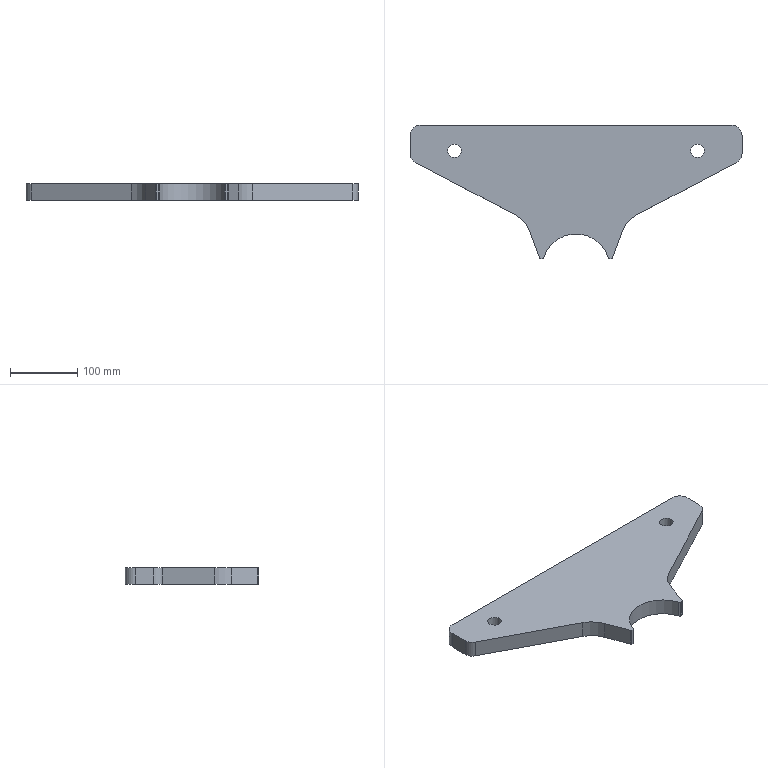Part | NX | features 压板 2 | 1 solid | 24 faces | box 492 x 197.84 x 25 mm | volume 1447958 mm3 | cylinder 13 | plane 11 | commonest cylinder face diameters 4 x4 30 x4 20 x2 90 x2 100 x1
STEP:
#1=CARTESIAN_POINT('',(190.,173.16,25.));
#2=VERTEX_POINT('',#1);
#3=CARTESIAN_POINT('',(180.,173.16,25.));
#4=DIRECTION('',(0.,0.,1.));
#5=DIRECTION('',(1.,0.,0.));
#6=AXIS2_PLACEMENT_3D('',#3,#4,#5);
#7=CIRCLE('',#6,10.);
#8=EDGE_CURVE('',#2,#2,#7,.T.);
#9=ORIENTED_EDGE('',*,*,#8,.F.);
#10=EDGE_LOOP('',(#9));
#11=FACE_BOUND('',#10,.T.);
#12=CARTESIAN_POINT('',(52.393,13.16,25.));
#13=VERTEX_POINT('',#12);
#14=CARTESIAN_POINT('',(54.273,14.476,25.));
#15=VERTEX_POINT('',#14);
#16=CARTESIAN_POINT('',(52.393,15.16,25.));
#17=DIRECTION('',(0.,0.,1.));
#18=DIRECTION('',(-1.,0.,0.));
#19=AXIS2_PLACEMENT_3D('',#16,#17,#18);
#20=CIRCLE('',#19,2.);
#21=EDGE_CURVE('',#13,#15,#20,.T.);
#22=ORIENTED_EDGE('',*,*,#21,.T.);
#23=CARTESIAN_POINT('',(68.526,53.635,25.));
#24=VERTEX_POINT('',#23);
#25=CARTESIAN_POINT('',(54.273,14.476,25.));
#26=DIRECTION('',(0.342,0.9397,0.));
#27=VECTOR('',#26,1000.);
#28=LINE('',#25,#27);
#29=EDGE_CURVE('',#15,#24,#28,.T.);
#30=ORIENTED_EDGE('',*,*,#29,.T.);
#31=CARTESIAN_POINT('',(89.903,78.092,25.));
#32=VERTEX_POINT('',#31);
#33=CARTESIAN_POINT('',(110.812,38.244,25.));
#34=DIRECTION('',(0.,0.,-1.));
#35=DIRECTION('',(-1.,0.,0.));
#36=AXIS2_PLACEMENT_3D('',#33,#34,#35);
#37=CIRCLE('',#36,45.);
#38=EDGE_CURVE('',#24,#32,#37,.T.);
#39=ORIENTED_EDGE('',*,*,#38,.T.);
#40=CARTESIAN_POINT('',(237.97,155.786,25.));
#41=VERTEX_POINT('',#40);
#42=CARTESIAN_POINT('',(237.97,155.786,25.));
#43=DIRECTION('',(0.8855,0.4646,0.));
#44=VECTOR('',#43,1000.);
#45=LINE('',#42,#44);
#46=EDGE_CURVE('',#32,#41,#45,.T.);
#47=ORIENTED_EDGE('',*,*,#46,.T.);
#48=CARTESIAN_POINT('',(246.,169.069,25.));
#49=VERTEX_POINT('',#48);
#50=CARTESIAN_POINT('',(231.,169.069,25.));
#51=DIRECTION('',(0.,0.,1.));
#52=DIRECTION('',(1.,0.,0.));
#53=AXIS2_PLACEMENT_3D('',#50,#51,#52);
#54=CIRCLE('',#53,15.);
#55=EDGE_CURVE('',#41,#49,#54,.T.);
#56=ORIENTED_EDGE('',*,*,#55,.T.);
#57=CARTESIAN_POINT('',(246.,196.,25.));
#58=VERTEX_POINT('',#57);
#59=CARTESIAN_POINT('',(246.,196.,25.));
#60=DIRECTION('',(0.,1.,0.));
#61=VECTOR('',#60,1000.);
#62=LINE('',#59,#61);
#63=EDGE_CURVE('',#49,#58,#62,.T.);
#64=ORIENTED_EDGE('',*,*,#63,.T.);
#65=CARTESIAN_POINT('',(231.,211.,25.));
#66=VERTEX_POINT('',#65);
#67=CARTESIAN_POINT('',(231.,196.,25.));
#68=DIRECTION('',(0.,0.,1.));
#69=DIRECTION('',(1.,0.,0.));
#70=AXIS2_PLACEMENT_3D('',#67,#68,#69);
#71=CIRCLE('',#70,15.);
#72=EDGE_CURVE('',#58,#66,#71,.T.);
#73=ORIENTED_EDGE('',*,*,#72,.T.);
#74=CARTESIAN_POINT('',(-231.,211.,25.));
#75=VERTEX_POINT('',#74);
#76=CARTESIAN_POINT('',(231.,211.,25.));
#77=DIRECTION('',(-1.,0.,0.));
#78=VECTOR('',#77,1000.);
#79=LINE('',#76,#78);
#80=EDGE_CURVE('',#66,#75,#79,.T.);
#81=ORIENTED_EDGE('',*,*,#80,.T.);
#82=CARTESIAN_POINT('',(-246.,196.,25.));
#83=VERTEX_POINT('',#82);
#84=CARTESIAN_POINT('',(-231.,196.,25.));
#85=DIRECTION('',(0.,0.,1.));
#86=DIRECTION('',(-1.,0.,0.));
#87=AXIS2_PLACEMENT_3D('',#84,#85,#86);
#88=CIRCLE('',#87,15.);
#89=EDGE_CURVE('',#75,#83,#88,.T.);
#90=ORIENTED_EDGE('',*,*,#89,.T.);
#91=CARTESIAN_POINT('',(-246.,169.069,25.));
#92=VERTEX_POINT('',#91);
#93=CARTESIAN_POINT('',(-246.,196.,25.));
#94=DIRECTION('',(0.,-1.,0.));
#95=VECTOR('',#94,1000.);
#96=LINE('',#93,#95);
#97=EDGE_CURVE('',#83,#92,#96,.T.);
#98=ORIENTED_EDGE('',*,*,#97,.T.);
#99=CARTESIAN_POINT('',(-237.97,155.786,25.));
#100=VERTEX_POINT('',#99);
#101=CARTESIAN_POINT('',(-231.,169.069,25.));
#102=DIRECTION('',(0.,0.,1.));
#103=DIRECTION('',(-1.,0.,0.));
#104=AXIS2_PLACEMENT_3D('',#101,#102,#103);
#105=CIRCLE('',#104,15.);
#106=EDGE_CURVE('',#92,#100,#105,.T.);
#107=ORIENTED_EDGE('',*,*,#106,.T.);
#108=CARTESIAN_POINT('',(-89.903,78.092,25.));
#109=VERTEX_POINT('',#108);
#110=CARTESIAN_POINT('',(-237.97,155.786,25.));
#111=DIRECTION('',(0.8855,-0.4646,0.));
#112=VECTOR('',#111,1000.);
#113=LINE('',#110,#112);
#114=EDGE_CURVE('',#100,#109,#113,.T.);
#115=ORIENTED_EDGE('',*,*,#114,.T.);
#116=CARTESIAN_POINT('',(-68.526,53.635,25.));
#117=VERTEX_POINT('',#116);
#118=CARTESIAN_POINT('',(-110.812,38.244,25.));
#119=DIRECTION('',(0.,0.,-1.));
#120=DIRECTION('',(1.,0.,0.));
#121=AXIS2_PLACEMENT_3D('',#118,#119,#120);
#122=CIRCLE('',#121,45.);
#123=EDGE_CURVE('',#109,#117,#122,.T.);
#124=ORIENTED_EDGE('',*,*,#123,.T.);
#125=CARTESIAN_POINT('',(-54.273,14.476,25.));
#126=VERTEX_POINT('',#125);
#127=CARTESIAN_POINT('',(-54.273,14.476,25.));
#128=DIRECTION('',(0.342,-0.9397,0.));
#129=VECTOR('',#128,1000.);
#130=LINE('',#127,#129);
#131=EDGE_CURVE('',#117,#126,#130,.T.);
#132=ORIENTED_EDGE('',*,*,#131,.T.);
#133=CARTESIAN_POINT('',(-52.393,13.16,25.));
#134=VERTEX_POINT('',#133);
#135=CARTESIAN_POINT('',(-52.393,15.16,25.));
#136=DIRECTION('',(0.,0.,1.));
#137=DIRECTION('',(1.,0.,0.));
#138=AXIS2_PLACEMENT_3D('',#135,#136,#137);
#139=CIRCLE('',#138,2.);
#140=EDGE_CURVE('',#126,#134,#139,.T.);
#141=ORIENTED_EDGE('',*,*,#140,.T.);
#142=CARTESIAN_POINT('',(-49.741,13.16,25.));
#143=VERTEX_POINT('',#142);
#144=CARTESIAN_POINT('',(-49.741,13.16,25.));
#145=DIRECTION('',(1.,0.,0.));
#146=VECTOR('',#145,1000.);
#147=LINE('',#144,#146);
#148=EDGE_CURVE('',#134,#143,#147,.T.);
#149=ORIENTED_EDGE('',*,*,#148,.T.);
#150=CARTESIAN_POINT('',(-47.828,14.577,25.));
#151=VERTEX_POINT('',#150);
#152=CARTESIAN_POINT('',(-49.741,15.16,25.));
#153=DIRECTION('',(0.,0.,1.));
#154=DIRECTION('',(1.,0.,0.));
#155=AXIS2_PLACEMENT_3D('',#152,#153,#154);
#156=CIRCLE('',#155,2.);
#157=EDGE_CURVE('',#143,#151,#156,.T.);
#158=ORIENTED_EDGE('',*,*,#157,.T.);
#159=CARTESIAN_POINT('',(47.828,14.577,25.));
#160=VERTEX_POINT('',#159);
#161=CARTESIAN_POINT('',(0.,0.,25.));
#162=DIRECTION('',(0.,0.,-1.));
#163=DIRECTION('',(1.,0.,0.));
#164=AXIS2_PLACEMENT_3D('',#161,#162,#163);
#165=CIRCLE('',#164,50.);
#166=EDGE_CURVE('',#151,#160,#165,.T.);
#167=ORIENTED_EDGE('',*,*,#166,.T.);
#168=CARTESIAN_POINT('',(49.741,13.16,25.));
#169=VERTEX_POINT('',#168);
#170=CARTESIAN_POINT('',(49.741,15.16,25.));
#171=DIRECTION('',(0.,0.,1.));
#172=DIRECTION('',(-1.,0.,0.));
#173=AXIS2_PLACEMENT_3D('',#170,#171,#172);
#174=CIRCLE('',#173,2.);
#175=EDGE_CURVE('',#160,#169,#174,.T.);
#176=ORIENTED_EDGE('',*,*,#175,.T.);
#177=CARTESIAN_POINT('',(49.741,13.16,25.));
#178=DIRECTION('',(1.,0.,0.));
#179=VECTOR('',#178,1000.);
#180=LINE('',#177,#179);
#181=EDGE_CURVE('',#169,#13,#180,.T.);
#182=ORIENTED_EDGE('',*,*,#181,.T.);
#183=EDGE_LOOP('',(#22,#30,#39,#47,#56,#64,#73,#81,#90,#98,#107,#115,#124,#132,#141,#149,#158,#167,#176,#182));
#184=FACE_BOUND('',#183,.T.);
#185=CARTESIAN_POINT('',(-190.,173.16,25.));
#186=VERTEX_POINT('',#185);
#187=CARTESIAN_POINT('',(-180.,173.16,25.));
#188=DIRECTION('',(0.,0.,1.));
#189=DIRECTION('',(-1.,0.,0.));
#190=AXIS2_PLACEMENT_3D('',#187,#188,#189);
#191=CIRCLE('',#190,10.);
#192=EDGE_CURVE('',#186,#186,#191,.T.);
#193=ORIENTED_EDGE('',*,*,#192,.F.);
#194=EDGE_LOOP('',(#193));
#195=FACE_BOUND('',#194,.T.);
#196=CARTESIAN_POINT('',(52.393,15.16,25.));
#197=DIRECTION('',(0.,0.,-1.));
#198=DIRECTION('',(-1.,0.,0.));
#199=AXIS2_PLACEMENT_3D('',#196,#197,#198);
#200=PLANE('',#199);
#201=ADVANCED_FACE('',(#11,#184,#195),#200,.F.);
#202=CARTESIAN_POINT('',(190.,173.16,0.));
#203=VERTEX_POINT('',#202);
#204=CARTESIAN_POINT('',(180.,173.16,0.));
#205=DIRECTION('',(0.,0.,1.));
#206=DIRECTION('',(1.,0.,0.));
#207=AXIS2_PLACEMENT_3D('',#204,#205,#206);
#208=CIRCLE('',#207,10.);
#209=EDGE_CURVE('',#203,#203,#208,.T.);
#210=ORIENTED_EDGE('',*,*,#209,.T.);
#211=EDGE_LOOP('',(#210));
#212=FACE_BOUND('',#211,.T.);
#213=CARTESIAN_POINT('',(52.393,13.16,0.));
#214=VERTEX_POINT('',#213);
#215=CARTESIAN_POINT('',(54.273,14.476,0.));
#216=VERTEX_POINT('',#215);
#217=CARTESIAN_POINT('',(52.393,15.16,0.));
#218=DIRECTION('',(0.,0.,1.));
#219=DIRECTION('',(-1.,0.,0.));
#220=AXIS2_PLACEMENT_3D('',#217,#218,#219);
#221=CIRCLE('',#220,2.);
#222=EDGE_CURVE('',#214,#216,#221,.T.);
#223=ORIENTED_EDGE('',*,*,#222,.F.);
#224=CARTESIAN_POINT('',(49.741,13.16,0.));
#225=VERTEX_POINT('',#224);
#226=CARTESIAN_POINT('',(49.741,13.16,0.));
#227=DIRECTION('',(1.,0.,0.));
#228=VECTOR('',#227,1000.);
#229=LINE('',#226,#228);
#230=EDGE_CURVE('',#225,#214,#229,.T.);
#231=ORIENTED_EDGE('',*,*,#230,.F.);
#232=CARTESIAN_POINT('',(47.828,14.577,0.));
#233=VERTEX_POINT('',#232);
#234=CARTESIAN_POINT('',(49.741,15.16,0.));
#235=DIRECTION('',(0.,0.,1.));
#236=DIRECTION('',(-1.,0.,0.));
#237=AXIS2_PLACEMENT_3D('',#234,#235,#236);
#238=CIRCLE('',#237,2.);
#239=EDGE_CURVE('',#233,#225,#238,.T.);
#240=ORIENTED_EDGE('',*,*,#239,.F.);
#241=CARTESIAN_POINT('',(-47.828,14.577,0.));
#242=VERTEX_POINT('',#241);
#243=CARTESIAN_POINT('',(0.,0.,0.));
#244=DIRECTION('',(0.,0.,-1.));
#245=DIRECTION('',(1.,0.,0.));
#246=AXIS2_PLACEMENT_3D('',#243,#244,#245);
#247=CIRCLE('',#246,50.);
#248=EDGE_CURVE('',#242,#233,#247,.T.);
#249=ORIENTED_EDGE('',*,*,#248,.F.);
#250=CARTESIAN_POINT('',(-49.741,13.16,0.));
#251=VERTEX_POINT('',#250);
#252=CARTESIAN_POINT('',(-49.741,15.16,0.));
#253=DIRECTION('',(0.,0.,1.));
#254=DIRECTION('',(1.,0.,0.));
#255=AXIS2_PLACEMENT_3D('',#252,#253,#254);
#256=CIRCLE('',#255,2.);
#257=EDGE_CURVE('',#251,#242,#256,.T.);
#258=ORIENTED_EDGE('',*,*,#257,.F.);
#259=CARTESIAN_POINT('',(-52.393,13.16,0.));
#260=VERTEX_POINT('',#259);
#261=CARTESIAN_POINT('',(-49.741,13.16,0.));
#262=DIRECTION('',(1.,0.,0.));
#263=VECTOR('',#262,1000.);
#264=LINE('',#261,#263);
#265=EDGE_CURVE('',#260,#251,#264,.T.);
#266=ORIENTED_EDGE('',*,*,#265,.F.);
#267=CARTESIAN_POINT('',(-54.273,14.476,0.));
#268=VERTEX_POINT('',#267);
#269=CARTESIAN_POINT('',(-52.393,15.16,0.));
#270=DIRECTION('',(0.,0.,1.));
#271=DIRECTION('',(1.,0.,0.));
#272=AXIS2_PLACEMENT_3D('',#269,#270,#271);
#273=CIRCLE('',#272,2.);
#274=EDGE_CURVE('',#268,#260,#273,.T.);
#275=ORIENTED_EDGE('',*,*,#274,.F.);
#276=CARTESIAN_POINT('',(-68.526,53.635,0.));
#277=VERTEX_POINT('',#276);
#278=CARTESIAN_POINT('',(-54.273,14.476,0.));
#279=DIRECTION('',(0.342,-0.9397,0.));
#280=VECTOR('',#279,1000.);
#281=LINE('',#278,#280);
#282=EDGE_CURVE('',#277,#268,#281,.T.);
#283=ORIENTED_EDGE('',*,*,#282,.F.);
#284=CARTESIAN_POINT('',(-89.903,78.092,0.));
#285=VERTEX_POINT('',#284);
#286=CARTESIAN_POINT('',(-110.812,38.244,0.));
#287=DIRECTION('',(0.,0.,-1.));
#288=DIRECTION('',(1.,0.,0.));
#289=AXIS2_PLACEMENT_3D('',#286,#287,#288);
#290=CIRCLE('',#289,45.);
#291=EDGE_CURVE('',#285,#277,#290,.T.);
#292=ORIENTED_EDGE('',*,*,#291,.F.);
#293=CARTESIAN_POINT('',(-237.97,155.786,0.));
#294=VERTEX_POINT('',#293);
#295=CARTESIAN_POINT('',(-237.97,155.786,0.));
#296=DIRECTION('',(0.8855,-0.4646,0.));
#297=VECTOR('',#296,1000.);
#298=LINE('',#295,#297);
#299=EDGE_CURVE('',#294,#285,#298,.T.);
#300=ORIENTED_EDGE('',*,*,#299,.F.);
#301=CARTESIAN_POINT('',(-246.,169.069,0.));
#302=VERTEX_POINT('',#301);
#303=CARTESIAN_POINT('',(-231.,169.069,0.));
#304=DIRECTION('',(0.,0.,1.));
#305=DIRECTION('',(-1.,0.,0.));
#306=AXIS2_PLACEMENT_3D('',#303,#304,#305);
#307=CIRCLE('',#306,15.);
#308=EDGE_CURVE('',#302,#294,#307,.T.);
#309=ORIENTED_EDGE('',*,*,#308,.F.);
#310=CARTESIAN_POINT('',(-246.,196.,0.));
#311=VERTEX_POINT('',#310);
#312=CARTESIAN_POINT('',(-246.,196.,0.));
#313=DIRECTION('',(0.,-1.,0.));
#314=VECTOR('',#313,1000.);
#315=LINE('',#312,#314);
#316=EDGE_CURVE('',#311,#302,#315,.T.);
#317=ORIENTED_EDGE('',*,*,#316,.F.);
#318=CARTESIAN_POINT('',(-231.,211.,0.));
#319=VERTEX_POINT('',#318);
#320=CARTESIAN_POINT('',(-231.,196.,0.));
#321=DIRECTION('',(0.,0.,1.));
#322=DIRECTION('',(-1.,0.,0.));
#323=AXIS2_PLACEMENT_3D('',#320,#321,#322);
#324=CIRCLE('',#323,15.);
#325=EDGE_CURVE('',#319,#311,#324,.T.);
#326=ORIENTED_EDGE('',*,*,#325,.F.);
#327=CARTESIAN_POINT('',(231.,211.,0.));
#328=VERTEX_POINT('',#327);
#329=CARTESIAN_POINT('',(231.,211.,0.));
#330=DIRECTION('',(-1.,0.,0.));
#331=VECTOR('',#330,1000.);
#332=LINE('',#329,#331);
#333=EDGE_CURVE('',#328,#319,#332,.T.);
#334=ORIENTED_EDGE('',*,*,#333,.F.);
#335=CARTESIAN_POINT('',(246.,196.,0.));
#336=VERTEX_POINT('',#335);
#337=CARTESIAN_POINT('',(231.,196.,0.));
#338=DIRECTION('',(0.,0.,1.));
#339=DIRECTION('',(1.,0.,0.));
#340=AXIS2_PLACEMENT_3D('',#337,#338,#339);
#341=CIRCLE('',#340,15.);
#342=EDGE_CURVE('',#336,#328,#341,.T.);
#343=ORIENTED_EDGE('',*,*,#342,.F.);
#344=CARTESIAN_POINT('',(246.,169.069,0.));
#345=VERTEX_POINT('',#344);
#346=CARTESIAN_POINT('',(246.,196.,0.));
#347=DIRECTION('',(0.,1.,0.));
#348=VECTOR('',#347,1000.);
#349=LINE('',#346,#348);
#350=EDGE_CURVE('',#345,#336,#349,.T.);
#351=ORIENTED_EDGE('',*,*,#350,.F.);
#352=CARTESIAN_POINT('',(237.97,155.786,0.));
#353=VERTEX_POINT('',#352);
#354=CARTESIAN_POINT('',(231.,169.069,0.));
#355=DIRECTION('',(0.,0.,1.));
#356=DIRECTION('',(1.,0.,0.));
#357=AXIS2_PLACEMENT_3D('',#354,#355,#356);
#358=CIRCLE('',#357,15.);
#359=EDGE_CURVE('',#353,#345,#358,.T.);
#360=ORIENTED_EDGE('',*,*,#359,.F.);
#361=CARTESIAN_POINT('',(89.903,78.092,0.));
#362=VERTEX_POINT('',#361);
#363=CARTESIAN_POINT('',(237.97,155.786,0.));
#364=DIRECTION('',(0.8855,0.4646,0.));
#365=VECTOR('',#364,1000.);
#366=LINE('',#363,#365);
#367=EDGE_CURVE('',#362,#353,#366,.T.);
#368=ORIENTED_EDGE('',*,*,#367,.F.);
#369=CARTESIAN_POINT('',(68.526,53.635,0.));
#370=VERTEX_POINT('',#369);
#371=CARTESIAN_POINT('',(110.812,38.244,0.));
#372=DIRECTION('',(0.,0.,-1.));
#373=DIRECTION('',(-1.,0.,0.));
#374=AXIS2_PLACEMENT_3D('',#371,#372,#373);
#375=CIRCLE('',#374,45.);
#376=EDGE_CURVE('',#370,#362,#375,.T.);
#377=ORIENTED_EDGE('',*,*,#376,.F.);
#378=CARTESIAN_POINT('',(54.273,14.476,0.));
#379=DIRECTION('',(0.342,0.9397,0.));
#380=VECTOR('',#379,1000.);
#381=LINE('',#378,#380);
#382=EDGE_CURVE('',#216,#370,#381,.T.);
#383=ORIENTED_EDGE('',*,*,#382,.F.);
#384=EDGE_LOOP('',(#223,#231,#240,#249,#258,#266,#275,#283,#292,#300,#309,#317,#326,#334,#343,#351,#360,#368,#377,#383));
#385=FACE_BOUND('',#384,.T.);
#386=CARTESIAN_POINT('',(-190.,173.16,0.));
#387=VERTEX_POINT('',#386);
#388=CARTESIAN_POINT('',(-180.,173.16,0.));
#389=DIRECTION('',(0.,0.,1.));
#390=DIRECTION('',(-1.,0.,0.));
#391=AXIS2_PLACEMENT_3D('',#388,#389,#390);
#392=CIRCLE('',#391,10.);
#393=EDGE_CURVE('',#387,#387,#392,.T.);
#394=ORIENTED_EDGE('',*,*,#393,.T.);
#395=EDGE_LOOP('',(#394));
#396=FACE_BOUND('',#395,.T.);
#397=CARTESIAN_POINT('',(52.393,15.16,0.));
#398=DIRECTION('',(0.,0.,-1.));
#399=DIRECTION('',(-1.,0.,0.));
#400=AXIS2_PLACEMENT_3D('',#397,#398,#399);
#401=PLANE('',#400);
#402=ADVANCED_FACE('',(#212,#385,#396),#401,.T.);
#403=ORIENTED_EDGE('',*,*,#222,.T.);
#404=CARTESIAN_POINT('',(54.273,14.476,25.));
#405=DIRECTION('',(0.,0.,-1.));
#406=VECTOR('',#405,1000.);
#407=LINE('',#404,#406);
#408=EDGE_CURVE('',#15,#216,#407,.T.);
#409=ORIENTED_EDGE('',*,*,#408,.F.);
#410=ORIENTED_EDGE('',*,*,#21,.F.);
#411=CARTESIAN_POINT('',(52.393,13.16,25.));
#412=DIRECTION('',(0.,0.,-1.));
#413=VECTOR('',#412,1000.);
#414=LINE('',#411,#413);
#415=EDGE_CURVE('',#13,#214,#414,.T.);
#416=ORIENTED_EDGE('',*,*,#415,.T.);
#417=EDGE_LOOP('',(#403,#409,#410,#416));
#418=FACE_BOUND('',#417,.T.);
#419=CARTESIAN_POINT('',(52.393,15.16,25.));
#420=DIRECTION('',(0.,0.,-1.));
#421=DIRECTION('',(-1.,0.,0.));
#422=AXIS2_PLACEMENT_3D('',#419,#420,#421);
#423=CYLINDRICAL_SURFACE('',#422,2.);
#424=ADVANCED_FACE('',(#418),#423,.T.);
#425=ORIENTED_EDGE('',*,*,#382,.T.);
#426=CARTESIAN_POINT('',(68.526,53.635,25.));
#427=DIRECTION('',(0.,0.,-1.));
#428=VECTOR('',#427,1000.);
#429=LINE('',#426,#428);
#430=EDGE_CURVE('',#24,#370,#429,.T.);
#431=ORIENTED_EDGE('',*,*,#430,.F.);
#432=ORIENTED_EDGE('',*,*,#29,.F.);
#433=ORIENTED_EDGE('',*,*,#408,.T.);
#434=EDGE_LOOP('',(#425,#431,#432,#433));
#435=FACE_BOUND('',#434,.T.);
#436=CARTESIAN_POINT('',(54.273,14.476,25.));
#437=DIRECTION('',(-0.9397,0.342,0.));
#438=DIRECTION('',(-0.342,-0.9397,0.));
#439=AXIS2_PLACEMENT_3D('',#436,#437,#438);
#440=PLANE('',#439);
#441=ADVANCED_FACE('',(#435),#440,.F.);
#442=ORIENTED_EDGE('',*,*,#376,.T.);
#443=CARTESIAN_POINT('',(89.903,78.092,25.));
#444=DIRECTION('',(0.,0.,-1.));
#445=VECTOR('',#444,1000.);
#446=LINE('',#443,#445);
#447=EDGE_CURVE('',#32,#362,#446,.T.);
#448=ORIENTED_EDGE('',*,*,#447,.F.);
#449=ORIENTED_EDGE('',*,*,#38,.F.);
#450=ORIENTED_EDGE('',*,*,#430,.T.);
#451=EDGE_LOOP('',(#442,#448,#449,#450));
#452=FACE_BOUND('',#451,.T.);
#453=CARTESIAN_POINT('',(110.812,38.244,25.));
#454=DIRECTION('',(0.,0.,-1.));
#455=DIRECTION('',(-1.,0.,0.));
#456=AXIS2_PLACEMENT_3D('',#453,#454,#455);
#457=CYLINDRICAL_SURFACE('',#456,45.);
#458=ADVANCED_FACE('',(#452),#457,.F.);
#459=ORIENTED_EDGE('',*,*,#367,.T.);
#460=CARTESIAN_POINT('',(237.97,155.786,25.));
#461=DIRECTION('',(0.,0.,-1.));
#462=VECTOR('',#461,1000.);
#463=LINE('',#460,#462);
#464=EDGE_CURVE('',#41,#353,#463,.T.);
#465=ORIENTED_EDGE('',*,*,#464,.F.);
#466=ORIENTED_EDGE('',*,*,#46,.F.);
#467=ORIENTED_EDGE('',*,*,#447,.T.);
#468=EDGE_LOOP('',(#459,#465,#466,#467));
#469=FACE_BOUND('',#468,.T.);
#470=CARTESIAN_POINT('',(237.97,155.786,25.));
#471=DIRECTION('',(-0.4646,0.8855,0.));
#472=DIRECTION('',(-0.8855,-0.4646,0.));
#473=AXIS2_PLACEMENT_3D('',#470,#471,#472);
#474=PLANE('',#473);
#475=ADVANCED_FACE('',(#469),#474,.F.);
#476=ORIENTED_EDGE('',*,*,#359,.T.);
#477=CARTESIAN_POINT('',(246.,169.069,25.));
#478=DIRECTION('',(0.,0.,-1.));
#479=VECTOR('',#478,1000.);
#480=LINE('',#477,#479);
#481=EDGE_CURVE('',#49,#345,#480,.T.);
#482=ORIENTED_EDGE('',*,*,#481,.F.);
#483=ORIENTED_EDGE('',*,*,#55,.F.);
#484=ORIENTED_EDGE('',*,*,#464,.T.);
#485=EDGE_LOOP('',(#476,#482,#483,#484));
#486=FACE_BOUND('',#485,.T.);
#487=CARTESIAN_POINT('',(231.,169.069,25.));
#488=DIRECTION('',(0.,0.,-1.));
#489=DIRECTION('',(-1.,0.,0.));
#490=AXIS2_PLACEMENT_3D('',#487,#488,#489);
#491=CYLINDRICAL_SURFACE('',#490,15.);
#492=ADVANCED_FACE('',(#486),#491,.T.);
#493=ORIENTED_EDGE('',*,*,#350,.T.);
#494=CARTESIAN_POINT('',(246.,196.,25.));
#495=DIRECTION('',(0.,0.,-1.));
#496=VECTOR('',#495,1000.);
#497=LINE('',#494,#496);
#498=EDGE_CURVE('',#58,#336,#497,.T.);
#499=ORIENTED_EDGE('',*,*,#498,.F.);
#500=ORIENTED_EDGE('',*,*,#63,.F.);
#501=ORIENTED_EDGE('',*,*,#481,.T.);
#502=EDGE_LOOP('',(#493,#499,#500,#501));
#503=FACE_BOUND('',#502,.T.);
#504=CARTESIAN_POINT('',(246.,196.,25.));
#505=DIRECTION('',(-1.,0.,0.));
#506=DIRECTION('',(0.,-1.,0.));
#507=AXIS2_PLACEMENT_3D('',#504,#505,#506);
#508=PLANE('',#507);
#509=ADVANCED_FACE('',(#503),#508,.F.);
#510=ORIENTED_EDGE('',*,*,#342,.T.);
#511=CARTESIAN_POINT('',(231.,211.,25.));
#512=DIRECTION('',(0.,0.,-1.));
#513=VECTOR('',#512,1000.);
#514=LINE('',#511,#513);
#515=EDGE_CURVE('',#66,#328,#514,.T.);
#516=ORIENTED_EDGE('',*,*,#515,.F.);
#517=ORIENTED_EDGE('',*,*,#72,.F.);
#518=ORIENTED_EDGE('',*,*,#498,.T.);
#519=EDGE_LOOP('',(#510,#516,#517,#518));
#520=FACE_BOUND('',#519,.T.);
#521=CARTESIAN_POINT('',(231.,196.,25.));
#522=DIRECTION('',(0.,0.,-1.));
#523=DIRECTION('',(-1.,0.,0.));
#524=AXIS2_PLACEMENT_3D('',#521,#522,#523);
#525=CYLINDRICAL_SURFACE('',#524,15.);
#526=ADVANCED_FACE('',(#520),#525,.T.);
#527=ORIENTED_EDGE('',*,*,#333,.T.);
#528=CARTESIAN_POINT('',(-231.,211.,25.));
#529=DIRECTION('',(0.,0.,-1.));
#530=VECTOR('',#529,1000.);
#531=LINE('',#528,#530);
#532=EDGE_CURVE('',#75,#319,#531,.T.);
#533=ORIENTED_EDGE('',*,*,#532,.F.);
#534=ORIENTED_EDGE('',*,*,#80,.F.);
#535=ORIENTED_EDGE('',*,*,#515,.T.);
#536=EDGE_LOOP('',(#527,#533,#534,#535));
#537=FACE_BOUND('',#536,.T.);
#538=CARTESIAN_POINT('',(231.,211.,25.));
#539=DIRECTION('',(0.,-1.,0.));
#540=DIRECTION('',(0.,0.,-1.));
#541=AXIS2_PLACEMENT_3D('',#538,#539,#540);
#542=PLANE('',#541);
#543=ADVANCED_FACE('',(#537),#542,.F.);
#544=ORIENTED_EDGE('',*,*,#325,.T.);
#545=CARTESIAN_POINT('',(-246.,196.,25.));
#546=DIRECTION('',(0.,0.,-1.));
#547=VECTOR('',#546,1000.);
#548=LINE('',#545,#547);
#549=EDGE_CURVE('',#83,#311,#548,.T.);
#550=ORIENTED_EDGE('',*,*,#549,.F.);
#551=ORIENTED_EDGE('',*,*,#89,.F.);
#552=ORIENTED_EDGE('',*,*,#532,.T.);
#553=EDGE_LOOP('',(#544,#550,#551,#552));
#554=FACE_BOUND('',#553,.T.);
#555=CARTESIAN_POINT('',(-231.,196.,25.));
#556=DIRECTION('',(0.,0.,-1.));
#557=DIRECTION('',(-1.,0.,0.));
#558=AXIS2_PLACEMENT_3D('',#555,#556,#557);
#559=CYLINDRICAL_SURFACE('',#558,15.);
#560=ADVANCED_FACE('',(#554),#559,.T.);
#561=ORIENTED_EDGE('',*,*,#316,.T.);
#562=CARTESIAN_POINT('',(-246.,169.069,25.));
#563=DIRECTION('',(0.,0.,-1.));
#564=VECTOR('',#563,1000.);
#565=LINE('',#562,#564);
#566=EDGE_CURVE('',#92,#302,#565,.T.);
#567=ORIENTED_EDGE('',*,*,#566,.F.);
#568=ORIENTED_EDGE('',*,*,#97,.F.);
#569=ORIENTED_EDGE('',*,*,#549,.T.);
#570=EDGE_LOOP('',(#561,#567,#568,#569));
#571=FACE_BOUND('',#570,.T.);
#572=CARTESIAN_POINT('',(-246.,196.,25.));
#573=DIRECTION('',(1.,0.,0.));
#574=DIRECTION('',(0.,1.,0.));
#575=AXIS2_PLACEMENT_3D('',#572,#573,#574);
#576=PLANE('',#575);
#577=ADVANCED_FACE('',(#571),#576,.F.);
#578=ORIENTED_EDGE('',*,*,#308,.T.);
#579=CARTESIAN_POINT('',(-237.97,155.786,25.));
#580=DIRECTION('',(0.,0.,-1.));
#581=VECTOR('',#580,1000.);
#582=LINE('',#579,#581);
#583=EDGE_CURVE('',#100,#294,#582,.T.);
#584=ORIENTED_EDGE('',*,*,#583,.F.);
#585=ORIENTED_EDGE('',*,*,#106,.F.);
#586=ORIENTED_EDGE('',*,*,#566,.T.);
#587=EDGE_LOOP('',(#578,#584,#585,#586));
#588=FACE_BOUND('',#587,.T.);
#589=CARTESIAN_POINT('',(-231.,169.069,25.));
#590=DIRECTION('',(0.,0.,-1.));
#591=DIRECTION('',(-1.,0.,0.));
#592=AXIS2_PLACEMENT_3D('',#589,#590,#591);
#593=CYLINDRICAL_SURFACE('',#592,15.);
#594=ADVANCED_FACE('',(#588),#593,.T.);
#595=ORIENTED_EDGE('',*,*,#299,.T.);
#596=CARTESIAN_POINT('',(-89.903,78.092,25.));
#597=DIRECTION('',(0.,0.,-1.));
#598=VECTOR('',#597,1000.);
#599=LINE('',#596,#598);
#600=EDGE_CURVE('',#109,#285,#599,.T.);
#601=ORIENTED_EDGE('',*,*,#600,.F.);
#602=ORIENTED_EDGE('',*,*,#114,.F.);
#603=ORIENTED_EDGE('',*,*,#583,.T.);
#604=EDGE_LOOP('',(#595,#601,#602,#603));
#605=FACE_BOUND('',#604,.T.);
#606=CARTESIAN_POINT('',(-237.97,155.786,25.));
#607=DIRECTION('',(0.4646,0.8855,0.));
#608=DIRECTION('',(-0.8855,0.4646,0.));
#609=AXIS2_PLACEMENT_3D('',#606,#607,#608);
#610=PLANE('',#609);
#611=ADVANCED_FACE('',(#605),#610,.F.);
#612=ORIENTED_EDGE('',*,*,#291,.T.);
#613=CARTESIAN_POINT('',(-68.526,53.635,25.));
#614=DIRECTION('',(0.,0.,-1.));
#615=VECTOR('',#614,1000.);
#616=LINE('',#613,#615);
#617=EDGE_CURVE('',#117,#277,#616,.T.);
#618=ORIENTED_EDGE('',*,*,#617,.F.);
#619=ORIENTED_EDGE('',*,*,#123,.F.);
#620=ORIENTED_EDGE('',*,*,#600,.T.);
#621=EDGE_LOOP('',(#612,#618,#619,#620));
#622=FACE_BOUND('',#621,.T.);
#623=CARTESIAN_POINT('',(-110.812,38.244,25.));
#624=DIRECTION('',(0.,0.,-1.));
#625=DIRECTION('',(-1.,0.,0.));
#626=AXIS2_PLACEMENT_3D('',#623,#624,#625);
#627=CYLINDRICAL_SURFACE('',#626,45.);
#628=ADVANCED_FACE('',(#622),#627,.F.);
#629=ORIENTED_EDGE('',*,*,#282,.T.);
#630=CARTESIAN_POINT('',(-54.273,14.476,25.));
#631=DIRECTION('',(0.,0.,-1.));
#632=VECTOR('',#631,1000.);
#633=LINE('',#630,#632);
#634=EDGE_CURVE('',#126,#268,#633,.T.);
#635=ORIENTED_EDGE('',*,*,#634,.F.);
#636=ORIENTED_EDGE('',*,*,#131,.F.);
#637=ORIENTED_EDGE('',*,*,#617,.T.);
#638=EDGE_LOOP('',(#629,#635,#636,#637));
#639=FACE_BOUND('',#638,.T.);
#640=CARTESIAN_POINT('',(-54.273,14.476,25.));
#641=DIRECTION('',(0.9397,0.342,0.));
#642=DIRECTION('',(-0.342,0.9397,0.));
#643=AXIS2_PLACEMENT_3D('',#640,#641,#642);
#644=PLANE('',#643);
#645=ADVANCED_FACE('',(#639),#644,.F.);
#646=ORIENTED_EDGE('',*,*,#274,.T.);
#647=CARTESIAN_POINT('',(-52.393,13.16,25.));
#648=DIRECTION('',(0.,0.,-1.));
#649=VECTOR('',#648,1000.);
#650=LINE('',#647,#649);
#651=EDGE_CURVE('',#134,#260,#650,.T.);
#652=ORIENTED_EDGE('',*,*,#651,.F.);
#653=ORIENTED_EDGE('',*,*,#140,.F.);
#654=ORIENTED_EDGE('',*,*,#634,.T.);
#655=EDGE_LOOP('',(#646,#652,#653,#654));
#656=FACE_BOUND('',#655,.T.);
#657=CARTESIAN_POINT('',(-52.393,15.16,25.));
#658=DIRECTION('',(0.,0.,-1.));
#659=DIRECTION('',(-1.,0.,0.));
#660=AXIS2_PLACEMENT_3D('',#657,#658,#659);
#661=CYLINDRICAL_SURFACE('',#660,2.);
#662=ADVANCED_FACE('',(#656),#661,.T.);
#663=ORIENTED_EDGE('',*,*,#265,.T.);
#664=CARTESIAN_POINT('',(-49.741,13.16,25.));
#665=DIRECTION('',(0.,0.,-1.));
#666=VECTOR('',#665,1000.);
#667=LINE('',#664,#666);
#668=EDGE_CURVE('',#143,#251,#667,.T.);
#669=ORIENTED_EDGE('',*,*,#668,.F.);
#670=ORIENTED_EDGE('',*,*,#148,.F.);
#671=ORIENTED_EDGE('',*,*,#651,.T.);
#672=EDGE_LOOP('',(#663,#669,#670,#671));
#673=FACE_BOUND('',#672,.T.);
#674=CARTESIAN_POINT('',(-49.741,13.16,25.));
#675=DIRECTION('',(0.,1.,0.));
#676=DIRECTION('',(0.,0.,1.));
#677=AXIS2_PLACEMENT_3D('',#674,#675,#676);
#678=PLANE('',#677);
#679=ADVANCED_FACE('',(#673),#678,.F.);
#680=ORIENTED_EDGE('',*,*,#257,.T.);
#681=CARTESIAN_POINT('',(-47.828,14.577,25.));
#682=DIRECTION('',(0.,0.,-1.));
#683=VECTOR('',#682,1000.);
#684=LINE('',#681,#683);
#685=EDGE_CURVE('',#151,#242,#684,.T.);
#686=ORIENTED_EDGE('',*,*,#685,.F.);
#687=ORIENTED_EDGE('',*,*,#157,.F.);
#688=ORIENTED_EDGE('',*,*,#668,.T.);
#689=EDGE_LOOP('',(#680,#686,#687,#688));
#690=FACE_BOUND('',#689,.T.);
#691=CARTESIAN_POINT('',(-49.741,15.16,25.));
#692=DIRECTION('',(0.,0.,-1.));
#693=DIRECTION('',(-1.,0.,0.));
#694=AXIS2_PLACEMENT_3D('',#691,#692,#693);
#695=CYLINDRICAL_SURFACE('',#694,2.);
#696=ADVANCED_FACE('',(#690),#695,.T.);
#697=ORIENTED_EDGE('',*,*,#248,.T.);
#698=CARTESIAN_POINT('',(47.828,14.577,25.));
#699=DIRECTION('',(0.,0.,-1.));
#700=VECTOR('',#699,1000.);
#701=LINE('',#698,#700);
#702=EDGE_CURVE('',#160,#233,#701,.T.);
#703=ORIENTED_EDGE('',*,*,#702,.F.);
#704=ORIENTED_EDGE('',*,*,#166,.F.);
#705=ORIENTED_EDGE('',*,*,#685,.T.);
#706=EDGE_LOOP('',(#697,#703,#704,#705));
#707=FACE_BOUND('',#706,.T.);
#708=CARTESIAN_POINT('',(0.,0.,25.));
#709=DIRECTION('',(0.,0.,-1.));
#710=DIRECTION('',(-1.,0.,0.));
#711=AXIS2_PLACEMENT_3D('',#708,#709,#710);
#712=CYLINDRICAL_SURFACE('',#711,50.);
#713=ADVANCED_FACE('',(#707),#712,.F.);
#714=ORIENTED_EDGE('',*,*,#239,.T.);
#715=CARTESIAN_POINT('',(49.741,13.16,25.));
#716=DIRECTION('',(0.,0.,-1.));
#717=VECTOR('',#716,1000.);
#718=LINE('',#715,#717);
#719=EDGE_CURVE('',#169,#225,#718,.T.);
#720=ORIENTED_EDGE('',*,*,#719,.F.);
#721=ORIENTED_EDGE('',*,*,#175,.F.);
#722=ORIENTED_EDGE('',*,*,#702,.T.);
#723=EDGE_LOOP('',(#714,#720,#721,#722));
#724=FACE_BOUND('',#723,.T.);
#725=CARTESIAN_POINT('',(49.741,15.16,25.));
#726=DIRECTION('',(0.,0.,-1.));
#727=DIRECTION('',(-1.,0.,0.));
#728=AXIS2_PLACEMENT_3D('',#725,#726,#727);
#729=CYLINDRICAL_SURFACE('',#728,2.);
#730=ADVANCED_FACE('',(#724),#729,.T.);
#731=ORIENTED_EDGE('',*,*,#230,.T.);
#732=ORIENTED_EDGE('',*,*,#415,.F.);
#733=ORIENTED_EDGE('',*,*,#181,.F.);
#734=ORIENTED_EDGE('',*,*,#719,.T.);
#735=EDGE_LOOP('',(#731,#732,#733,#734));
#736=FACE_BOUND('',#735,.T.);
#737=CARTESIAN_POINT('',(49.741,13.16,25.));
#738=DIRECTION('',(0.,1.,0.));
#739=DIRECTION('',(0.,0.,1.));
#740=AXIS2_PLACEMENT_3D('',#737,#738,#739);
#741=PLANE('',#740);
#742=ADVANCED_FACE('',(#736),#741,.F.);
#743=ORIENTED_EDGE('',*,*,#8,.T.);
#744=EDGE_LOOP('',(#743));
#745=FACE_BOUND('',#744,.T.);
#746=ORIENTED_EDGE('',*,*,#209,.F.);
#747=EDGE_LOOP('',(#746));
#748=FACE_BOUND('',#747,.T.);
#749=CARTESIAN_POINT('',(180.,173.16,25.));
#750=DIRECTION('',(0.,0.,-1.));
#751=DIRECTION('',(-1.,0.,0.));
#752=AXIS2_PLACEMENT_3D('',#749,#750,#751);
#753=CYLINDRICAL_SURFACE('',#752,10.);
#754=ADVANCED_FACE('',(#745,#748),#753,.F.);
#755=ORIENTED_EDGE('',*,*,#192,.T.);
#756=EDGE_LOOP('',(#755));
#757=FACE_BOUND('',#756,.T.);
#758=ORIENTED_EDGE('',*,*,#393,.F.);
#759=EDGE_LOOP('',(#758));
#760=FACE_BOUND('',#759,.T.);
#761=CARTESIAN_POINT('',(-180.,173.16,25.));
#762=DIRECTION('',(0.,0.,-1.));
#763=DIRECTION('',(-1.,0.,0.));
#764=AXIS2_PLACEMENT_3D('',#761,#762,#763);
#765=CYLINDRICAL_SURFACE('',#764,10.);
#766=ADVANCED_FACE('',(#757,#760),#765,.F.);
#767=CLOSED_SHELL('',(#201,#402,#424,#441,#458,#475,#492,#509,#526,#543,#560,#577,#594,#611,#628,#645,#662,#679,#696,#713,#730,#742,#754,#766));
#768=MANIFOLD_SOLID_BREP('',#767);
#769=(LENGTH_UNIT()NAMED_UNIT(*)SI_UNIT(.MILLI.,.METRE.));
#770=UNCERTAINTY_MEASURE_WITH_UNIT(LENGTH_MEASURE(0.00001),#769,'','');
#771=(NAMED_UNIT(*)PLANE_ANGLE_UNIT()SI_UNIT($,.RADIAN.));
#772=(NAMED_UNIT(*)SI_UNIT($,.STERADIAN.)SOLID_ANGLE_UNIT());
#773=(GEOMETRIC_REPRESENTATION_CONTEXT(3)GLOBAL_UNCERTAINTY_ASSIGNED_CONTEXT((#770))GLOBAL_UNIT_ASSIGNED_CONTEXT((#769,#771,#772))REPRESENTATION_CONTEXT('',''));
#774=ADVANCED_BREP_SHAPE_REPRESENTATION('',(#768),#773);